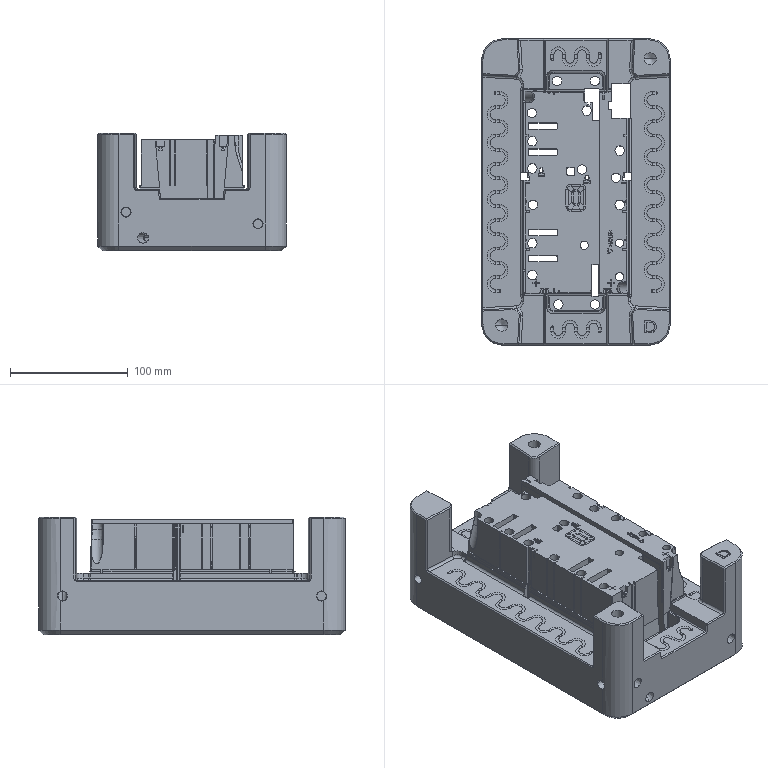Part | Creo | 1 solid | 2174 faces | box 160 x 260 x 100 mm | volume 2325601 mm3 | plane 959 | cylinder 574 | other 396 | cone 146 | torus 49 | spline 30 | sphere 20 | commonest cylinder face diameters 8 x101 6 x91 0.603 x59 1 x51 4 x48 12 x35